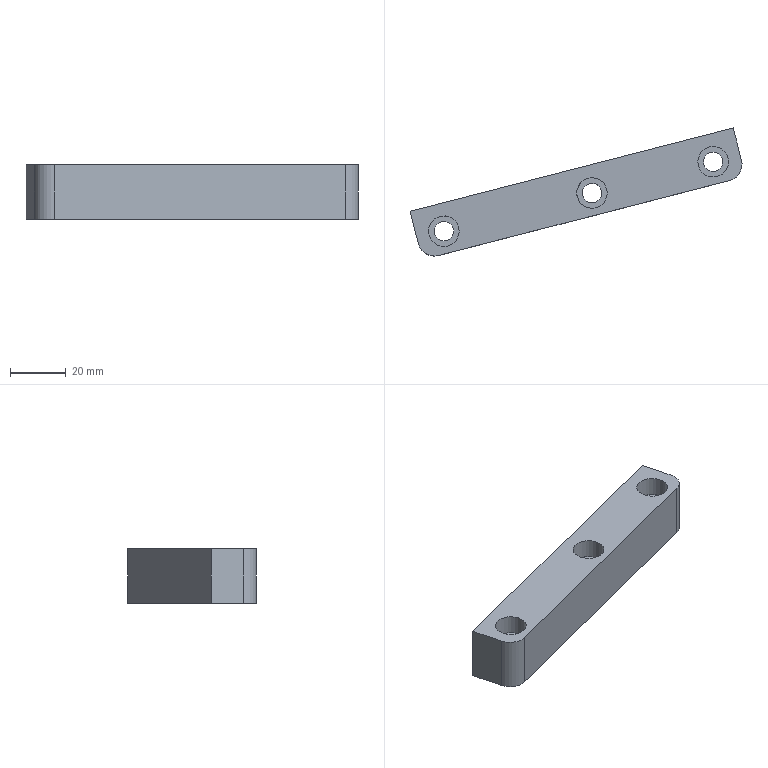Part | STEP file | 车灯-后视镜_id142_x_t | 1 solid | 17 faces | box 119.383 x 46.093 x 19.5 mm | volume 38380 mm3 | plane 9 | cylinder 8 | commonest cylinder face diameters 7 x3 11 x3 12 x2
STEP:
#1=CARTESIAN_POINT('',(-171.661,-173.865,-19.147));
#2=VERTEX_POINT('',#1);
#3=CARTESIAN_POINT('',(-168.597,-172.172,-19.147));
#4=DIRECTION('',(0.,0.,-1.));
#5=DIRECTION('',(-0.8752,-0.4837,0.));
#6=AXIS2_PLACEMENT_3D('',#3,#4,#5);
#7=CIRCLE('',#6,3.5);
#8=EDGE_CURVE('',#2,#2,#7,.T.);
#9=ORIENTED_EDGE('',*,*,#8,.F.);
#10=EDGE_LOOP('',(#9));
#11=FACE_BOUND('',#10,.T.);
#12=CARTESIAN_POINT('',(-118.84,-158.435,-19.147));
#13=VERTEX_POINT('',#12);
#14=CARTESIAN_POINT('',(-115.34,-158.435,-19.147));
#15=DIRECTION('',(0.,0.,-1.));
#16=DIRECTION('',(-1.,0.,0.));
#17=AXIS2_PLACEMENT_3D('',#14,#15,#16);
#18=CIRCLE('',#17,3.5);
#19=EDGE_CURVE('',#13,#13,#18,.T.);
#20=ORIENTED_EDGE('',*,*,#19,.F.);
#21=EDGE_LOOP('',(#20));
#22=FACE_BOUND('',#21,.T.);
#23=CARTESIAN_POINT('',(-74.83,-148.888,-19.147));
#24=VERTEX_POINT('',#23);
#25=CARTESIAN_POINT('',(-71.767,-147.195,-19.147));
#26=DIRECTION('',(0.,0.,-1.));
#27=DIRECTION('',(-0.8752,-0.4837,0.));
#28=AXIS2_PLACEMENT_3D('',#25,#26,#27);
#29=CIRCLE('',#28,3.5);
#30=EDGE_CURVE('',#24,#24,#29,.T.);
#31=ORIENTED_EDGE('',*,*,#30,.F.);
#32=EDGE_LOOP('',(#31));
#33=FACE_BOUND('',#32,.T.);
#34=CARTESIAN_POINT('',(-61.585,-146.635,-19.147));
#35=VERTEX_POINT('',#34);
#36=CARTESIAN_POINT('',(-64.582,-135.015,-19.147));
#37=VERTEX_POINT('',#36);
#38=CARTESIAN_POINT('',(-60.086,-152.444,-19.147));
#39=DIRECTION('',(-0.2498,0.9683,0.));
#40=VECTOR('',#39,1.);
#41=LINE('',#38,#40);
#42=EDGE_CURVE('',#35,#37,#41,.T.);
#43=ORIENTED_EDGE('',*,*,#42,.F.);
#44=CARTESIAN_POINT('',(-65.896,-153.943,-19.147));
#45=VERTEX_POINT('',#44);
#46=CARTESIAN_POINT('',(-67.395,-148.133,-19.147));
#47=DIRECTION('',(0.,0.,-1.));
#48=DIRECTION('',(1.,0.,0.));
#49=AXIS2_PLACEMENT_3D('',#46,#47,#48);
#50=CIRCLE('',#49,6.);
#51=EDGE_CURVE('',#35,#45,#50,.T.);
#52=ORIENTED_EDGE('',*,*,#51,.T.);
#53=CARTESIAN_POINT('',(-170.472,-180.917,-19.147));
#54=VERTEX_POINT('',#53);
#55=CARTESIAN_POINT('',(-156.917,-177.421,-19.147));
#56=DIRECTION('',(0.9683,0.2498,0.));
#57=VECTOR('',#56,1.);
#58=LINE('',#55,#57);
#59=EDGE_CURVE('',#54,#45,#58,.T.);
#60=ORIENTED_EDGE('',*,*,#59,.F.);
#61=CARTESIAN_POINT('',(-177.781,-176.606,-19.147));
#62=VERTEX_POINT('',#61);
#63=CARTESIAN_POINT('',(-171.971,-175.108,-19.147));
#64=DIRECTION('',(0.,0.,-1.));
#65=DIRECTION('',(1.,0.,0.));
#66=AXIS2_PLACEMENT_3D('',#63,#64,#65);
#67=CIRCLE('',#66,6.);
#68=EDGE_CURVE('',#54,#62,#67,.T.);
#69=ORIENTED_EDGE('',*,*,#68,.T.);
#70=CARTESIAN_POINT('',(-180.778,-164.986,-19.147));
#71=VERTEX_POINT('',#70);
#72=CARTESIAN_POINT('',(-176.282,-182.416,-19.147));
#73=DIRECTION('',(-0.2498,0.9683,0.));
#74=VECTOR('',#73,1.);
#75=LINE('',#72,#74);
#76=EDGE_CURVE('',#62,#71,#75,.T.);
#77=ORIENTED_EDGE('',*,*,#76,.T.);
#78=CARTESIAN_POINT('',(-161.413,-159.991,-19.147));
#79=DIRECTION('',(0.9683,0.2498,0.));
#80=VECTOR('',#79,1.);
#81=LINE('',#78,#80);
#82=EDGE_CURVE('',#71,#37,#81,.T.);
#83=ORIENTED_EDGE('',*,*,#82,.T.);
#84=EDGE_LOOP('',(#43,#52,#60,#69,#77,#83));
#85=FACE_BOUND('',#84,.T.);
#86=CARTESIAN_POINT('',(-156.917,-177.421,-19.147));
#87=DIRECTION('',(0.,0.,1.));
#88=DIRECTION('',(1.,0.,0.));
#89=AXIS2_PLACEMENT_3D('',#86,#87,#88);
#90=PLANE('',#89);
#91=ADVANCED_FACE('',(#11,#22,#33,#85),#90,.F.);
#92=ORIENTED_EDGE('',*,*,#76,.F.);
#93=CARTESIAN_POINT('',(-177.781,-176.606,0.3528));
#94=VERTEX_POINT('',#93);
#95=CARTESIAN_POINT('',(-177.781,-176.606,-10.327));
#96=DIRECTION('',(0.,0.,1.));
#97=VECTOR('',#96,1.);
#98=LINE('',#95,#97);
#99=EDGE_CURVE('',#62,#94,#98,.T.);
#100=ORIENTED_EDGE('',*,*,#99,.T.);
#101=CARTESIAN_POINT('',(-180.778,-164.986,0.3528));
#102=VERTEX_POINT('',#101);
#103=CARTESIAN_POINT('',(-183.276,-155.303,0.3528));
#104=DIRECTION('',(-0.2498,0.9683,0.));
#105=VECTOR('',#104,1.);
#106=LINE('',#103,#105);
#107=EDGE_CURVE('',#94,#102,#106,.T.);
#108=ORIENTED_EDGE('',*,*,#107,.T.);
#109=CARTESIAN_POINT('',(-180.778,-164.986,-10.147));
#110=DIRECTION('',(0.,0.,1.));
#111=VECTOR('',#110,1.);
#112=LINE('',#109,#111);
#113=EDGE_CURVE('',#71,#102,#112,.T.);
#114=ORIENTED_EDGE('',*,*,#113,.F.);
#115=EDGE_LOOP('',(#92,#100,#108,#114));
#116=FACE_OUTER_BOUND('',#115,.T.);
#117=CARTESIAN_POINT('',(-183.276,-155.303,-10.327));
#118=DIRECTION('',(-0.9683,-0.2498,0.));
#119=DIRECTION('',(0.,0.,1.));
#120=AXIS2_PLACEMENT_3D('',#117,#118,#119);
#121=PLANE('',#120);
#122=ADVANCED_FACE('',(#116),#121,.T.);
#123=CARTESIAN_POINT('',(-163.783,-169.512,0.3528));
#124=VERTEX_POINT('',#123);
#125=CARTESIAN_POINT('',(-168.597,-172.172,0.3528));
#126=DIRECTION('',(0.,0.,1.));
#127=DIRECTION('',(0.8752,0.4837,0.));
#128=AXIS2_PLACEMENT_3D('',#125,#126,#127);
#129=CIRCLE('',#128,5.5);
#130=EDGE_CURVE('',#124,#124,#129,.T.);
#131=ORIENTED_EDGE('',*,*,#130,.F.);
#132=EDGE_LOOP('',(#131));
#133=FACE_BOUND('',#132,.T.);
#134=CARTESIAN_POINT('',(-109.84,-158.435,0.3528));
#135=VERTEX_POINT('',#134);
#136=CARTESIAN_POINT('',(-115.34,-158.435,0.3528));
#137=DIRECTION('',(0.,0.,1.));
#138=DIRECTION('',(1.,0.,0.));
#139=AXIS2_PLACEMENT_3D('',#136,#137,#138);
#140=CIRCLE('',#139,5.5);
#141=EDGE_CURVE('',#135,#135,#140,.T.);
#142=ORIENTED_EDGE('',*,*,#141,.F.);
#143=EDGE_LOOP('',(#142));
#144=FACE_BOUND('',#143,.T.);
#145=CARTESIAN_POINT('',(-66.953,-144.535,0.3528));
#146=VERTEX_POINT('',#145);
#147=CARTESIAN_POINT('',(-71.767,-147.195,0.3528));
#148=DIRECTION('',(0.,0.,1.));
#149=DIRECTION('',(0.8752,0.4837,0.));
#150=AXIS2_PLACEMENT_3D('',#147,#148,#149);
#151=CIRCLE('',#150,5.5);
#152=EDGE_CURVE('',#146,#146,#151,.T.);
#153=ORIENTED_EDGE('',*,*,#152,.F.);
#154=EDGE_LOOP('',(#153));
#155=FACE_BOUND('',#154,.T.);
#156=CARTESIAN_POINT('',(-170.472,-180.917,0.3528));
#157=VERTEX_POINT('',#156);
#158=CARTESIAN_POINT('',(-65.896,-153.943,0.3528));
#159=VERTEX_POINT('',#158);
#160=CARTESIAN_POINT('',(33.12,-128.403,0.3528));
#161=DIRECTION('',(0.9683,0.2498,0.));
#162=VECTOR('',#161,1.);
#163=LINE('',#160,#162);
#164=EDGE_CURVE('',#157,#159,#163,.T.);
#165=ORIENTED_EDGE('',*,*,#164,.T.);
#166=CARTESIAN_POINT('',(-61.585,-146.635,0.3528));
#167=VERTEX_POINT('',#166);
#168=CARTESIAN_POINT('',(-67.395,-148.133,0.3528));
#169=DIRECTION('',(0.,0.,1.));
#170=DIRECTION('',(1.,0.,0.));
#171=AXIS2_PLACEMENT_3D('',#168,#169,#170);
#172=CIRCLE('',#171,6.);
#173=EDGE_CURVE('',#159,#167,#172,.T.);
#174=ORIENTED_EDGE('',*,*,#173,.T.);
#175=CARTESIAN_POINT('',(-64.582,-135.015,0.3528));
#176=VERTEX_POINT('',#175);
#177=CARTESIAN_POINT('',(-60.086,-152.444,0.3528));
#178=DIRECTION('',(-0.2498,0.9683,0.));
#179=VECTOR('',#178,1.);
#180=LINE('',#177,#179);
#181=EDGE_CURVE('',#167,#176,#180,.T.);
#182=ORIENTED_EDGE('',*,*,#181,.T.);
#183=CARTESIAN_POINT('',(28.624,-110.973,0.3528));
#184=DIRECTION('',(0.9683,0.2498,0.));
#185=VECTOR('',#184,1.);
#186=LINE('',#183,#185);
#187=EDGE_CURVE('',#102,#176,#186,.T.);
#188=ORIENTED_EDGE('',*,*,#187,.F.);
#189=ORIENTED_EDGE('',*,*,#107,.F.);
#190=CARTESIAN_POINT('',(-171.971,-175.108,0.3528));
#191=DIRECTION('',(0.,0.,1.));
#192=DIRECTION('',(1.,0.,0.));
#193=AXIS2_PLACEMENT_3D('',#190,#191,#192);
#194=CIRCLE('',#193,6.);
#195=EDGE_CURVE('',#94,#157,#194,.T.);
#196=ORIENTED_EDGE('',*,*,#195,.T.);
#197=EDGE_LOOP('',(#165,#174,#182,#188,#189,#196));
#198=FACE_BOUND('',#197,.T.);
#199=CARTESIAN_POINT('',(0.,0.,0.3528));
#200=DIRECTION('',(0.,0.,1.));
#201=DIRECTION('',(1.,0.,0.));
#202=AXIS2_PLACEMENT_3D('',#199,#200,#201);
#203=PLANE('',#202);
#204=ADVANCED_FACE('',(#133,#144,#155,#198),#203,.T.);
#205=ORIENTED_EDGE('',*,*,#181,.F.);
#206=CARTESIAN_POINT('',(-61.585,-146.635,-19.147));
#207=DIRECTION('',(0.,0.,-1.));
#208=VECTOR('',#207,1.);
#209=LINE('',#206,#208);
#210=EDGE_CURVE('',#167,#35,#209,.T.);
#211=ORIENTED_EDGE('',*,*,#210,.T.);
#212=ORIENTED_EDGE('',*,*,#42,.T.);
#213=CARTESIAN_POINT('',(-64.582,-135.015,-10.147));
#214=DIRECTION('',(0.,0.,1.));
#215=VECTOR('',#214,1.);
#216=LINE('',#213,#215);
#217=EDGE_CURVE('',#37,#176,#216,.T.);
#218=ORIENTED_EDGE('',*,*,#217,.T.);
#219=EDGE_LOOP('',(#205,#211,#212,#218));
#220=FACE_OUTER_BOUND('',#219,.T.);
#221=CARTESIAN_POINT('',(-60.086,-152.444,-10.147));
#222=DIRECTION('',(-0.9683,-0.2498,0.));
#223=DIRECTION('',(0.2498,-0.9683,0.));
#224=AXIS2_PLACEMENT_3D('',#221,#222,#223);
#225=PLANE('',#224);
#226=ADVANCED_FACE('',(#220),#225,.F.);
#227=ORIENTED_EDGE('',*,*,#59,.T.);
#228=CARTESIAN_POINT('',(-65.896,-153.943,0.7455));
#229=DIRECTION('',(0.,0.,1.));
#230=VECTOR('',#229,1.);
#231=LINE('',#228,#230);
#232=EDGE_CURVE('',#45,#159,#231,.T.);
#233=ORIENTED_EDGE('',*,*,#232,.T.);
#234=ORIENTED_EDGE('',*,*,#164,.F.);
#235=CARTESIAN_POINT('',(-170.472,-180.917,-10.147));
#236=DIRECTION('',(0.,0.,-1.));
#237=VECTOR('',#236,1.);
#238=LINE('',#235,#237);
#239=EDGE_CURVE('',#157,#54,#238,.T.);
#240=ORIENTED_EDGE('',*,*,#239,.T.);
#241=EDGE_LOOP('',(#227,#233,#234,#240));
#242=FACE_OUTER_BOUND('',#241,.T.);
#243=CARTESIAN_POINT('',(-108.501,-164.933,-10.147));
#244=DIRECTION('',(0.2498,-0.9683,0.));
#245=DIRECTION('',(0.,0.,-1.));
#246=AXIS2_PLACEMENT_3D('',#243,#244,#245);
#247=PLANE('',#246);
#248=ADVANCED_FACE('',(#242),#247,.T.);
#249=ORIENTED_EDGE('',*,*,#82,.F.);
#250=ORIENTED_EDGE('',*,*,#113,.T.);
#251=ORIENTED_EDGE('',*,*,#187,.T.);
#252=ORIENTED_EDGE('',*,*,#217,.F.);
#253=EDGE_LOOP('',(#249,#250,#251,#252));
#254=FACE_OUTER_BOUND('',#253,.T.);
#255=CARTESIAN_POINT('',(-112.997,-147.503,-10.147));
#256=DIRECTION('',(0.2498,-0.9683,0.));
#257=DIRECTION('',(0.,0.,-1.));
#258=AXIS2_PLACEMENT_3D('',#255,#256,#257);
#259=PLANE('',#258);
#260=ADVANCED_FACE('',(#254),#259,.F.);
#261=ORIENTED_EDGE('',*,*,#51,.F.);
#262=ORIENTED_EDGE('',*,*,#210,.F.);
#263=ORIENTED_EDGE('',*,*,#173,.F.);
#264=ORIENTED_EDGE('',*,*,#232,.F.);
#265=EDGE_LOOP('',(#261,#262,#263,#264));
#266=FACE_OUTER_BOUND('',#265,.T.);
#267=CARTESIAN_POINT('',(-67.395,-148.133,-10.147));
#268=DIRECTION('',(0.,0.,-1.));
#269=DIRECTION('',(-1.,0.,0.));
#270=AXIS2_PLACEMENT_3D('',#267,#268,#269);
#271=CYLINDRICAL_SURFACE('',#270,6.);
#272=ADVANCED_FACE('',(#266),#271,.T.);
#273=ORIENTED_EDGE('',*,*,#68,.F.);
#274=ORIENTED_EDGE('',*,*,#239,.F.);
#275=ORIENTED_EDGE('',*,*,#195,.F.);
#276=ORIENTED_EDGE('',*,*,#99,.F.);
#277=EDGE_LOOP('',(#273,#274,#275,#276));
#278=FACE_OUTER_BOUND('',#277,.T.);
#279=CARTESIAN_POINT('',(-171.971,-175.108,-10.327));
#280=DIRECTION('',(0.,0.,1.));
#281=DIRECTION('',(1.,0.,0.));
#282=AXIS2_PLACEMENT_3D('',#279,#280,#281);
#283=CYLINDRICAL_SURFACE('',#282,6.);
#284=ADVANCED_FACE('',(#278),#283,.T.);
#285=CARTESIAN_POINT('',(-74.83,-148.888,-6.647));
#286=VERTEX_POINT('',#285);
#287=CARTESIAN_POINT('',(-71.767,-147.195,-6.647));
#288=DIRECTION('',(0.,0.,-1.));
#289=DIRECTION('',(-0.8752,-0.4837,0.));
#290=AXIS2_PLACEMENT_3D('',#287,#288,#289);
#291=CIRCLE('',#290,3.5);
#292=EDGE_CURVE('',#286,#286,#291,.T.);
#293=ORIENTED_EDGE('',*,*,#292,.F.);
#294=EDGE_LOOP('',(#293));
#295=FACE_BOUND('',#294,.T.);
#296=ORIENTED_EDGE('',*,*,#30,.T.);
#297=EDGE_LOOP('',(#296));
#298=FACE_BOUND('',#297,.T.);
#299=CARTESIAN_POINT('',(-71.767,-147.195,-19.147));
#300=DIRECTION('',(0.,0.,1.));
#301=DIRECTION('',(-0.8752,-0.4837,0.));
#302=AXIS2_PLACEMENT_3D('',#299,#300,#301);
#303=CYLINDRICAL_SURFACE('',#302,3.5);
#304=ADVANCED_FACE('',(#295,#298),#303,.F.);
#305=ORIENTED_EDGE('',*,*,#292,.T.);
#306=EDGE_LOOP('',(#305));
#307=FACE_BOUND('',#306,.T.);
#308=CARTESIAN_POINT('',(-76.58,-149.856,-6.647));
#309=VERTEX_POINT('',#308);
#310=CARTESIAN_POINT('',(-71.767,-147.195,-6.647));
#311=DIRECTION('',(0.,0.,-1.));
#312=DIRECTION('',(-0.8752,-0.4837,0.));
#313=AXIS2_PLACEMENT_3D('',#310,#311,#312);
#314=CIRCLE('',#313,5.5);
#315=EDGE_CURVE('',#309,#309,#314,.T.);
#316=ORIENTED_EDGE('',*,*,#315,.F.);
#317=EDGE_LOOP('',(#316));
#318=FACE_BOUND('',#317,.T.);
#319=CARTESIAN_POINT('',(-71.767,-147.195,-6.647));
#320=DIRECTION('',(0.,0.,-1.));
#321=DIRECTION('',(0.8752,0.4837,0.));
#322=AXIS2_PLACEMENT_3D('',#319,#320,#321);
#323=PLANE('',#322);
#324=ADVANCED_FACE('',(#307,#318),#323,.F.);
#325=ORIENTED_EDGE('',*,*,#315,.T.);
#326=EDGE_LOOP('',(#325));
#327=FACE_BOUND('',#326,.T.);
#328=ORIENTED_EDGE('',*,*,#152,.T.);
#329=EDGE_LOOP('',(#328));
#330=FACE_BOUND('',#329,.T.);
#331=CARTESIAN_POINT('',(-71.767,-147.195,0.3528));
#332=DIRECTION('',(0.,0.,-1.));
#333=DIRECTION('',(0.8752,0.4837,0.));
#334=AXIS2_PLACEMENT_3D('',#331,#332,#333);
#335=CYLINDRICAL_SURFACE('',#334,5.5);
#336=ADVANCED_FACE('',(#327,#330),#335,.F.);
#337=CARTESIAN_POINT('',(-118.404,-160.128,-6.647));
#338=VERTEX_POINT('',#337);
#339=CARTESIAN_POINT('',(-115.34,-158.435,-6.647));
#340=DIRECTION('',(0.,0.,-1.));
#341=DIRECTION('',(-0.8752,-0.4837,0.));
#342=AXIS2_PLACEMENT_3D('',#339,#340,#341);
#343=CIRCLE('',#342,3.5);
#344=EDGE_CURVE('',#338,#338,#343,.T.);
#345=ORIENTED_EDGE('',*,*,#344,.F.);
#346=EDGE_LOOP('',(#345));
#347=FACE_BOUND('',#346,.T.);
#348=ORIENTED_EDGE('',*,*,#19,.T.);
#349=EDGE_LOOP('',(#348));
#350=FACE_BOUND('',#349,.T.);
#351=CARTESIAN_POINT('',(-115.34,-158.435,-19.147));
#352=DIRECTION('',(0.,0.,1.));
#353=DIRECTION('',(-0.8752,-0.4837,0.));
#354=AXIS2_PLACEMENT_3D('',#351,#352,#353);
#355=CYLINDRICAL_SURFACE('',#354,3.5);
#356=ADVANCED_FACE('',(#347,#350),#355,.F.);
#357=ORIENTED_EDGE('',*,*,#344,.T.);
#358=EDGE_LOOP('',(#357));
#359=FACE_BOUND('',#358,.T.);
#360=CARTESIAN_POINT('',(-120.154,-161.095,-6.647));
#361=VERTEX_POINT('',#360);
#362=CARTESIAN_POINT('',(-115.34,-158.435,-6.647));
#363=DIRECTION('',(0.,0.,-1.));
#364=DIRECTION('',(-0.8752,-0.4837,0.));
#365=AXIS2_PLACEMENT_3D('',#362,#363,#364);
#366=CIRCLE('',#365,5.5);
#367=EDGE_CURVE('',#361,#361,#366,.T.);
#368=ORIENTED_EDGE('',*,*,#367,.F.);
#369=EDGE_LOOP('',(#368));
#370=FACE_BOUND('',#369,.T.);
#371=CARTESIAN_POINT('',(-115.34,-158.435,-6.647));
#372=DIRECTION('',(0.,0.,-1.));
#373=DIRECTION('',(0.8752,0.4837,0.));
#374=AXIS2_PLACEMENT_3D('',#371,#372,#373);
#375=PLANE('',#374);
#376=ADVANCED_FACE('',(#359,#370),#375,.F.);
#377=ORIENTED_EDGE('',*,*,#367,.T.);
#378=EDGE_LOOP('',(#377));
#379=FACE_BOUND('',#378,.T.);
#380=ORIENTED_EDGE('',*,*,#141,.T.);
#381=EDGE_LOOP('',(#380));
#382=FACE_BOUND('',#381,.T.);
#383=CARTESIAN_POINT('',(-115.34,-158.435,0.3528));
#384=DIRECTION('',(0.,0.,-1.));
#385=DIRECTION('',(0.8752,0.4837,0.));
#386=AXIS2_PLACEMENT_3D('',#383,#384,#385);
#387=CYLINDRICAL_SURFACE('',#386,5.5);
#388=ADVANCED_FACE('',(#379,#382),#387,.F.);
#389=CARTESIAN_POINT('',(-171.661,-173.865,-6.647));
#390=VERTEX_POINT('',#389);
#391=CARTESIAN_POINT('',(-168.597,-172.172,-6.647));
#392=DIRECTION('',(0.,0.,-1.));
#393=DIRECTION('',(-0.8752,-0.4837,0.));
#394=AXIS2_PLACEMENT_3D('',#391,#392,#393);
#395=CIRCLE('',#394,3.5);
#396=EDGE_CURVE('',#390,#390,#395,.T.);
#397=ORIENTED_EDGE('',*,*,#396,.F.);
#398=EDGE_LOOP('',(#397));
#399=FACE_BOUND('',#398,.T.);
#400=ORIENTED_EDGE('',*,*,#8,.T.);
#401=EDGE_LOOP('',(#400));
#402=FACE_BOUND('',#401,.T.);
#403=CARTESIAN_POINT('',(-168.597,-172.172,-19.147));
#404=DIRECTION('',(0.,0.,1.));
#405=DIRECTION('',(-0.8752,-0.4837,0.));
#406=AXIS2_PLACEMENT_3D('',#403,#404,#405);
#407=CYLINDRICAL_SURFACE('',#406,3.5);
#408=ADVANCED_FACE('',(#399,#402),#407,.F.);
#409=ORIENTED_EDGE('',*,*,#396,.T.);
#410=EDGE_LOOP('',(#409));
#411=FACE_BOUND('',#410,.T.);
#412=CARTESIAN_POINT('',(-173.411,-174.832,-6.647));
#413=VERTEX_POINT('',#412);
#414=CARTESIAN_POINT('',(-168.597,-172.172,-6.647));
#415=DIRECTION('',(0.,0.,-1.));
#416=DIRECTION('',(-0.8752,-0.4837,0.));
#417=AXIS2_PLACEMENT_3D('',#414,#415,#416);
#418=CIRCLE('',#417,5.5);
#419=EDGE_CURVE('',#413,#413,#418,.T.);
#420=ORIENTED_EDGE('',*,*,#419,.F.);
#421=EDGE_LOOP('',(#420));
#422=FACE_BOUND('',#421,.T.);
#423=CARTESIAN_POINT('',(-168.597,-172.172,-6.647));
#424=DIRECTION('',(0.,0.,-1.));
#425=DIRECTION('',(0.8752,0.4837,0.));
#426=AXIS2_PLACEMENT_3D('',#423,#424,#425);
#427=PLANE('',#426);
#428=ADVANCED_FACE('',(#411,#422),#427,.F.);
#429=ORIENTED_EDGE('',*,*,#419,.T.);
#430=EDGE_LOOP('',(#429));
#431=FACE_BOUND('',#430,.T.);
#432=ORIENTED_EDGE('',*,*,#130,.T.);
#433=EDGE_LOOP('',(#432));
#434=FACE_BOUND('',#433,.T.);
#435=CARTESIAN_POINT('',(-168.597,-172.172,0.3528));
#436=DIRECTION('',(0.,0.,-1.));
#437=DIRECTION('',(0.8752,0.4837,0.));
#438=AXIS2_PLACEMENT_3D('',#435,#436,#437);
#439=CYLINDRICAL_SURFACE('',#438,5.5);
#440=ADVANCED_FACE('',(#431,#434),#439,.F.);
#441=CLOSED_SHELL('',(#91,#122,#204,#226,#248,#260,#272,#284,#304,#324,#336,#356,#376,#388,#408,#428,#440));
#442=MANIFOLD_SOLID_BREP('',#441);
#443=(LENGTH_UNIT()NAMED_UNIT(*)SI_UNIT(.MILLI.,.METRE.));
#444=UNCERTAINTY_MEASURE_WITH_UNIT(LENGTH_MEASURE(0.00002),#443,'','');
#445=(NAMED_UNIT(*)PLANE_ANGLE_UNIT()SI_UNIT($,.RADIAN.));
#446=PLANE_ANGLE_MEASURE_WITH_UNIT(PLANE_ANGLE_MEASURE(0.01745),#445);
#447=DIMENSIONAL_EXPONENTS(0.,0.,0.,0.,0.,0.,0.);
#448=(CONVERSION_BASED_UNIT('DEGREE',#446)NAMED_UNIT(#447)PLANE_ANGLE_UNIT());
#449=(NAMED_UNIT(*)SI_UNIT($,.STERADIAN.)SOLID_ANGLE_UNIT());
#450=(GEOMETRIC_REPRESENTATION_CONTEXT(3)GLOBAL_UNCERTAINTY_ASSIGNED_CONTEXT((#444))GLOBAL_UNIT_ASSIGNED_CONTEXT((#443,#448,#449))REPRESENTATION_CONTEXT('',''));
#451=ADVANCED_BREP_SHAPE_REPRESENTATION('',(#442),#450);